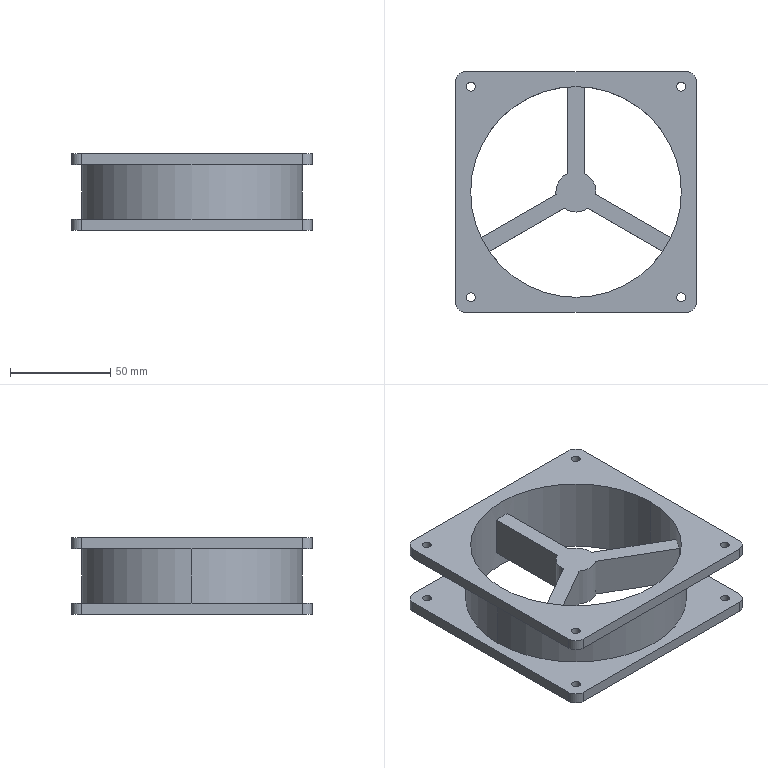Part | STEP file | Axial fan 1238A2MBL | 1 solid | 52 faces | box 120 x 120 x 38 mm | volume 111801 mm3 | cylinder 32 | plane 20 | commonest cylinder face diameters 4.5 x16 10 x8 20 x4 105 x2 110 x2